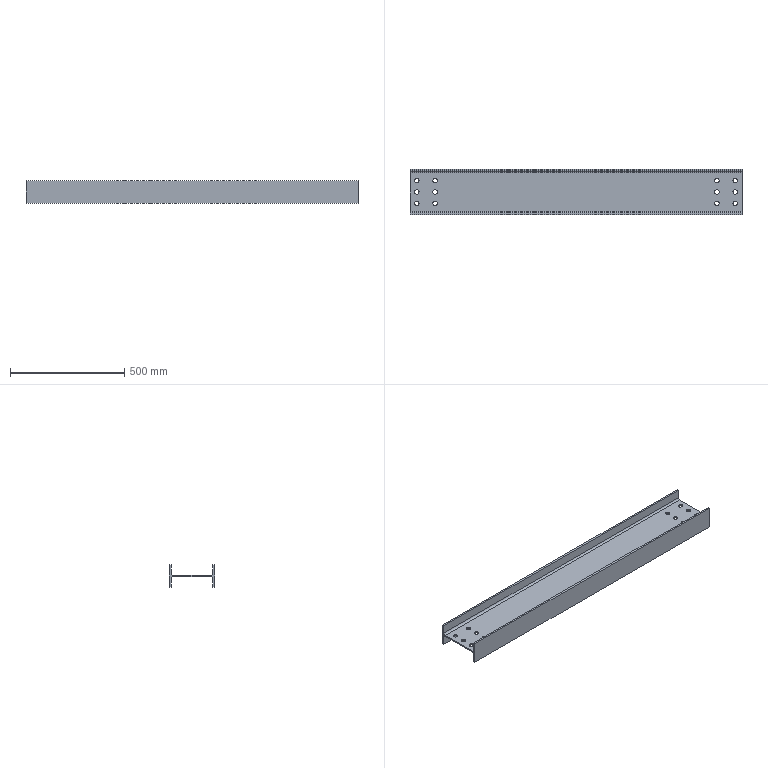Part | STEP file | 粉仓楼梯通道主梁1主体-200×100_Default<As Machined> | 1 solid | 42 faces | box 1455 x 200 x 100 mm | volume 3861682 mm3 | cylinder 28 | plane 14 | commonest cylinder face diameters 19 x24 16 x4